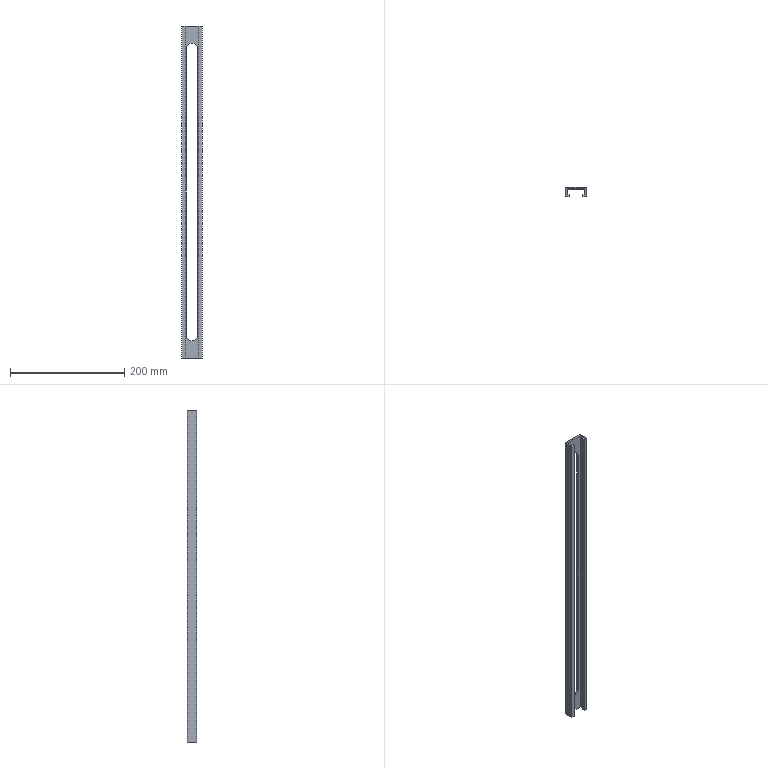Part | SolidWorks | features ICE 2, Extrusion 1 | 1 solid | 19 faces | box 36 x 16 x 580 mm | volume 87378 mm3 | plane 16 | cylinder 3 | commonest cylinder face diameters 20 x3
STEP:
#1=CARTESIAN_POINT('',(0.,13.,-260.));
#2=VERTEX_POINT('',#1);
#3=CARTESIAN_POINT('',(10.,13.,-250.));
#4=VERTEX_POINT('',#3);
#5=CARTESIAN_POINT('',(0.,13.,-250.));
#6=DIRECTION('',(0.,-1.,0.));
#7=DIRECTION('',(0.,0.,-1.));
#8=AXIS2_PLACEMENT_3D('',#5,#6,#7);
#9=CIRCLE('',#8,10.);
#10=EDGE_CURVE('',#2,#4,#9,.T.);
#11=ORIENTED_EDGE('',*,*,#10,.F.);
#12=CARTESIAN_POINT('',(0.,10.,-260.));
#13=VERTEX_POINT('',#12);
#14=CARTESIAN_POINT('',(0.,13.,-260.));
#15=DIRECTION('',(0.,-1.,0.));
#16=VECTOR('',#15,1000.);
#17=LINE('',#14,#16);
#18=EDGE_CURVE('',#2,#13,#17,.T.);
#19=ORIENTED_EDGE('',*,*,#18,.T.);
#20=CARTESIAN_POINT('',(10.,10.,-250.));
#21=VERTEX_POINT('',#20);
#22=CARTESIAN_POINT('',(0.,10.,-250.));
#23=DIRECTION('',(0.,-1.,0.));
#24=DIRECTION('',(0.,0.,-1.));
#25=AXIS2_PLACEMENT_3D('',#22,#23,#24);
#26=CIRCLE('',#25,10.);
#27=EDGE_CURVE('',#13,#21,#26,.T.);
#28=ORIENTED_EDGE('',*,*,#27,.T.);
#29=CARTESIAN_POINT('',(10.,13.,-250.));
#30=DIRECTION('',(0.,-1.,0.));
#31=VECTOR('',#30,1000.);
#32=LINE('',#29,#31);
#33=EDGE_CURVE('',#4,#21,#32,.T.);
#34=ORIENTED_EDGE('',*,*,#33,.F.);
#35=EDGE_LOOP('',(#11,#19,#28,#34));
#36=FACE_OUTER_BOUND('',#35,.T.);
#37=CARTESIAN_POINT('',(0.,13.,-250.));
#38=DIRECTION('',(0.,-1.,0.));
#39=DIRECTION('',(0.,0.,-1.));
#40=AXIS2_PLACEMENT_3D('',#37,#38,#39);
#41=CYLINDRICAL_SURFACE('',#40,10.);
#42=ADVANCED_FACE('',(#36),#41,.F.);
#43=CARTESIAN_POINT('',(12.,-3.,290.));
#44=VERTEX_POINT('',#43);
#45=CARTESIAN_POINT('',(18.,-3.,290.));
#46=VERTEX_POINT('',#45);
#47=CARTESIAN_POINT('',(-18.,-3.,290.));
#48=DIRECTION('',(1.,0.,0.));
#49=VECTOR('',#48,1000.);
#50=LINE('',#47,#49);
#51=EDGE_CURVE('',#44,#46,#50,.T.);
#52=ORIENTED_EDGE('',*,*,#51,.F.);
#53=CARTESIAN_POINT('',(12.,-3.,-290.));
#54=VERTEX_POINT('',#53);
#55=CARTESIAN_POINT('',(12.,-3.,290.));
#56=DIRECTION('',(0.,0.,-1.));
#57=VECTOR('',#56,1000.);
#58=LINE('',#55,#57);
#59=EDGE_CURVE('',#44,#54,#58,.T.);
#60=ORIENTED_EDGE('',*,*,#59,.T.);
#61=CARTESIAN_POINT('',(18.,-3.,-290.));
#62=VERTEX_POINT('',#61);
#63=CARTESIAN_POINT('',(18.,-3.,-290.));
#64=DIRECTION('',(-1.,0.,0.));
#65=VECTOR('',#64,1000.);
#66=LINE('',#63,#65);
#67=EDGE_CURVE('',#62,#54,#66,.T.);
#68=ORIENTED_EDGE('',*,*,#67,.F.);
#69=CARTESIAN_POINT('',(18.,-3.,290.));
#70=DIRECTION('',(0.,0.,-1.));
#71=VECTOR('',#70,1000.);
#72=LINE('',#69,#71);
#73=EDGE_CURVE('',#46,#62,#72,.T.);
#74=ORIENTED_EDGE('',*,*,#73,.F.);
#75=EDGE_LOOP('',(#52,#60,#68,#74));
#76=FACE_OUTER_BOUND('',#75,.T.);
#77=CARTESIAN_POINT('',(0.,-3.,0.));
#78=DIRECTION('',(0.,1.,0.));
#79=DIRECTION('',(0.,0.,1.));
#80=AXIS2_PLACEMENT_3D('',#77,#78,#79);
#81=PLANE('',#80);
#82=ADVANCED_FACE('',(#76),#81,.F.);
#83=CARTESIAN_POINT('',(-18.,13.,-290.));
#84=VERTEX_POINT('',#83);
#85=CARTESIAN_POINT('',(-18.,13.,290.));
#86=VERTEX_POINT('',#85);
#87=CARTESIAN_POINT('',(-18.,13.,-290.));
#88=DIRECTION('',(0.,0.,1.));
#89=VECTOR('',#88,1000.);
#90=LINE('',#87,#89);
#91=EDGE_CURVE('',#84,#86,#90,.T.);
#92=ORIENTED_EDGE('',*,*,#91,.F.);
#93=CARTESIAN_POINT('',(-18.,-3.,-290.));
#94=VERTEX_POINT('',#93);
#95=CARTESIAN_POINT('',(-18.,-3.,-290.));
#96=DIRECTION('',(0.,1.,0.));
#97=VECTOR('',#96,1000.);
#98=LINE('',#95,#97);
#99=EDGE_CURVE('',#94,#84,#98,.T.);
#100=ORIENTED_EDGE('',*,*,#99,.F.);
#101=CARTESIAN_POINT('',(-18.,-3.,290.));
#102=VERTEX_POINT('',#101);
#103=CARTESIAN_POINT('',(-18.,-3.,-290.));
#104=DIRECTION('',(0.,0.,1.));
#105=VECTOR('',#104,1000.);
#106=LINE('',#103,#105);
#107=EDGE_CURVE('',#94,#102,#106,.T.);
#108=ORIENTED_EDGE('',*,*,#107,.T.);
#109=CARTESIAN_POINT('',(-18.,-3.,290.));
#110=DIRECTION('',(0.,1.,0.));
#111=VECTOR('',#110,1000.);
#112=LINE('',#109,#111);
#113=EDGE_CURVE('',#102,#86,#112,.T.);
#114=ORIENTED_EDGE('',*,*,#113,.T.);
#115=EDGE_LOOP('',(#92,#100,#108,#114));
#116=FACE_OUTER_BOUND('',#115,.T.);
#117=CARTESIAN_POINT('',(-18.,-3.,-290.));
#118=DIRECTION('',(-1.,0.,0.));
#119=DIRECTION('',(0.,0.,1.));
#120=AXIS2_PLACEMENT_3D('',#117,#118,#119);
#121=PLANE('',#120);
#122=ADVANCED_FACE('',(#116),#121,.T.);
#123=CARTESIAN_POINT('',(12.,0.,-290.));
#124=VERTEX_POINT('',#123);
#125=CARTESIAN_POINT('',(12.,0.,-290.));
#126=DIRECTION('',(0.,-1.,0.));
#127=VECTOR('',#126,1000.);
#128=LINE('',#125,#127);
#129=EDGE_CURVE('',#124,#54,#128,.T.);
#130=ORIENTED_EDGE('',*,*,#129,.F.);
#131=CARTESIAN_POINT('',(15.,0.,-290.));
#132=VERTEX_POINT('',#131);
#133=CARTESIAN_POINT('',(15.,0.,-290.));
#134=DIRECTION('',(-1.,0.,0.));
#135=VECTOR('',#134,1000.);
#136=LINE('',#133,#135);
#137=EDGE_CURVE('',#132,#124,#136,.T.);
#138=ORIENTED_EDGE('',*,*,#137,.F.);
#139=CARTESIAN_POINT('',(15.,10.,-290.));
#140=VERTEX_POINT('',#139);
#141=CARTESIAN_POINT('',(15.,10.,-290.));
#142=DIRECTION('',(0.,-1.,0.));
#143=VECTOR('',#142,1000.);
#144=LINE('',#141,#143);
#145=EDGE_CURVE('',#140,#132,#144,.T.);
#146=ORIENTED_EDGE('',*,*,#145,.F.);
#147=CARTESIAN_POINT('',(-15.,10.,-290.));
#148=VERTEX_POINT('',#147);
#149=CARTESIAN_POINT('',(-15.,10.,-290.));
#150=DIRECTION('',(1.,0.,0.));
#151=VECTOR('',#150,1000.);
#152=LINE('',#149,#151);
#153=EDGE_CURVE('',#148,#140,#152,.T.);
#154=ORIENTED_EDGE('',*,*,#153,.F.);
#155=CARTESIAN_POINT('',(-15.,0.,-290.));
#156=VERTEX_POINT('',#155);
#157=CARTESIAN_POINT('',(-15.,0.,-290.));
#158=DIRECTION('',(0.,1.,0.));
#159=VECTOR('',#158,1000.);
#160=LINE('',#157,#159);
#161=EDGE_CURVE('',#156,#148,#160,.T.);
#162=ORIENTED_EDGE('',*,*,#161,.F.);
#163=CARTESIAN_POINT('',(-12.,0.,-290.));
#164=VERTEX_POINT('',#163);
#165=CARTESIAN_POINT('',(-12.,0.,-290.));
#166=DIRECTION('',(-1.,0.,0.));
#167=VECTOR('',#166,1000.);
#168=LINE('',#165,#167);
#169=EDGE_CURVE('',#164,#156,#168,.T.);
#170=ORIENTED_EDGE('',*,*,#169,.F.);
#171=CARTESIAN_POINT('',(-12.,-3.,-290.));
#172=VERTEX_POINT('',#171);
#173=CARTESIAN_POINT('',(-12.,-3.,-290.));
#174=DIRECTION('',(0.,1.,0.));
#175=VECTOR('',#174,1000.);
#176=LINE('',#173,#175);
#177=EDGE_CURVE('',#172,#164,#176,.T.);
#178=ORIENTED_EDGE('',*,*,#177,.F.);
#179=CARTESIAN_POINT('',(18.,-3.,-290.));
#180=DIRECTION('',(-1.,0.,0.));
#181=VECTOR('',#180,1000.);
#182=LINE('',#179,#181);
#183=EDGE_CURVE('',#172,#94,#182,.T.);
#184=ORIENTED_EDGE('',*,*,#183,.T.);
#185=ORIENTED_EDGE('',*,*,#99,.T.);
#186=CARTESIAN_POINT('',(18.,13.,-290.));
#187=VERTEX_POINT('',#186);
#188=CARTESIAN_POINT('',(18.,13.,-290.));
#189=DIRECTION('',(-1.,0.,0.));
#190=VECTOR('',#189,1000.);
#191=LINE('',#188,#190);
#192=EDGE_CURVE('',#187,#84,#191,.T.);
#193=ORIENTED_EDGE('',*,*,#192,.F.);
#194=CARTESIAN_POINT('',(18.,-3.,-290.));
#195=DIRECTION('',(0.,1.,0.));
#196=VECTOR('',#195,1000.);
#197=LINE('',#194,#196);
#198=EDGE_CURVE('',#62,#187,#197,.T.);
#199=ORIENTED_EDGE('',*,*,#198,.F.);
#200=ORIENTED_EDGE('',*,*,#67,.T.);
#201=EDGE_LOOP('',(#130,#138,#146,#154,#162,#170,#178,#184,#185,#193,#199,#200));
#202=FACE_OUTER_BOUND('',#201,.T.);
#203=CARTESIAN_POINT('',(18.,-3.,-290.));
#204=DIRECTION('',(0.,0.,-1.));
#205=DIRECTION('',(-1.,0.,0.));
#206=AXIS2_PLACEMENT_3D('',#203,#204,#205);
#207=PLANE('',#206);
#208=ADVANCED_FACE('',(#202),#207,.T.);
#209=CARTESIAN_POINT('',(18.,13.,290.));
#210=VERTEX_POINT('',#209);
#211=CARTESIAN_POINT('',(18.,13.,290.));
#212=DIRECTION('',(0.,0.,-1.));
#213=VECTOR('',#212,1000.);
#214=LINE('',#211,#213);
#215=EDGE_CURVE('',#210,#187,#214,.T.);
#216=ORIENTED_EDGE('',*,*,#215,.F.);
#217=CARTESIAN_POINT('',(18.,-3.,290.));
#218=DIRECTION('',(0.,1.,0.));
#219=VECTOR('',#218,1000.);
#220=LINE('',#217,#219);
#221=EDGE_CURVE('',#46,#210,#220,.T.);
#222=ORIENTED_EDGE('',*,*,#221,.F.);
#223=ORIENTED_EDGE('',*,*,#73,.T.);
#224=ORIENTED_EDGE('',*,*,#198,.T.);
#225=EDGE_LOOP('',(#216,#222,#223,#224));
#226=FACE_OUTER_BOUND('',#225,.T.);
#227=CARTESIAN_POINT('',(18.,-3.,290.));
#228=DIRECTION('',(1.,0.,0.));
#229=DIRECTION('',(0.,0.,-1.));
#230=AXIS2_PLACEMENT_3D('',#227,#228,#229);
#231=PLANE('',#230);
#232=ADVANCED_FACE('',(#226),#231,.T.);
#233=CARTESIAN_POINT('',(12.,0.,290.));
#234=VERTEX_POINT('',#233);
#235=CARTESIAN_POINT('',(12.,0.,290.));
#236=DIRECTION('',(0.,-1.,0.));
#237=VECTOR('',#236,1000.);
#238=LINE('',#235,#237);
#239=EDGE_CURVE('',#234,#44,#238,.T.);
#240=ORIENTED_EDGE('',*,*,#239,.T.);
#241=ORIENTED_EDGE('',*,*,#51,.T.);
#242=ORIENTED_EDGE('',*,*,#221,.T.);
#243=CARTESIAN_POINT('',(-18.,13.,290.));
#244=DIRECTION('',(1.,0.,0.));
#245=VECTOR('',#244,1000.);
#246=LINE('',#243,#245);
#247=EDGE_CURVE('',#86,#210,#246,.T.);
#248=ORIENTED_EDGE('',*,*,#247,.F.);
#249=ORIENTED_EDGE('',*,*,#113,.F.);
#250=CARTESIAN_POINT('',(-12.,-3.,290.));
#251=VERTEX_POINT('',#250);
#252=CARTESIAN_POINT('',(-18.,-3.,290.));
#253=DIRECTION('',(1.,0.,0.));
#254=VECTOR('',#253,1000.);
#255=LINE('',#252,#254);
#256=EDGE_CURVE('',#102,#251,#255,.T.);
#257=ORIENTED_EDGE('',*,*,#256,.T.);
#258=CARTESIAN_POINT('',(-12.,0.,290.));
#259=VERTEX_POINT('',#258);
#260=CARTESIAN_POINT('',(-12.,-3.,290.));
#261=DIRECTION('',(0.,1.,0.));
#262=VECTOR('',#261,1000.);
#263=LINE('',#260,#262);
#264=EDGE_CURVE('',#251,#259,#263,.T.);
#265=ORIENTED_EDGE('',*,*,#264,.T.);
#266=CARTESIAN_POINT('',(-15.,0.,290.));
#267=VERTEX_POINT('',#266);
#268=CARTESIAN_POINT('',(-12.,0.,290.));
#269=DIRECTION('',(-1.,0.,0.));
#270=VECTOR('',#269,1000.);
#271=LINE('',#268,#270);
#272=EDGE_CURVE('',#259,#267,#271,.T.);
#273=ORIENTED_EDGE('',*,*,#272,.T.);
#274=CARTESIAN_POINT('',(-15.,10.,290.));
#275=VERTEX_POINT('',#274);
#276=CARTESIAN_POINT('',(-15.,0.,290.));
#277=DIRECTION('',(0.,1.,0.));
#278=VECTOR('',#277,1000.);
#279=LINE('',#276,#278);
#280=EDGE_CURVE('',#267,#275,#279,.T.);
#281=ORIENTED_EDGE('',*,*,#280,.T.);
#282=CARTESIAN_POINT('',(15.,10.,290.));
#283=VERTEX_POINT('',#282);
#284=CARTESIAN_POINT('',(-15.,10.,290.));
#285=DIRECTION('',(1.,0.,0.));
#286=VECTOR('',#285,1000.);
#287=LINE('',#284,#286);
#288=EDGE_CURVE('',#275,#283,#287,.T.);
#289=ORIENTED_EDGE('',*,*,#288,.T.);
#290=CARTESIAN_POINT('',(15.,0.,290.));
#291=VERTEX_POINT('',#290);
#292=CARTESIAN_POINT('',(15.,10.,290.));
#293=DIRECTION('',(0.,-1.,0.));
#294=VECTOR('',#293,1000.);
#295=LINE('',#292,#294);
#296=EDGE_CURVE('',#283,#291,#295,.T.);
#297=ORIENTED_EDGE('',*,*,#296,.T.);
#298=CARTESIAN_POINT('',(15.,0.,290.));
#299=DIRECTION('',(-1.,0.,0.));
#300=VECTOR('',#299,1000.);
#301=LINE('',#298,#300);
#302=EDGE_CURVE('',#291,#234,#301,.T.);
#303=ORIENTED_EDGE('',*,*,#302,.T.);
#304=EDGE_LOOP('',(#240,#241,#242,#248,#249,#257,#265,#273,#281,#289,#297,#303));
#305=FACE_OUTER_BOUND('',#304,.T.);
#306=CARTESIAN_POINT('',(-18.,-3.,290.));
#307=DIRECTION('',(0.,0.,1.));
#308=DIRECTION('',(1.,0.,0.));
#309=AXIS2_PLACEMENT_3D('',#306,#307,#308);
#310=PLANE('',#309);
#311=ADVANCED_FACE('',(#305),#310,.T.);
#312=ORIENTED_EDGE('',*,*,#183,.F.);
#313=CARTESIAN_POINT('',(-12.,-3.,290.));
#314=DIRECTION('',(0.,0.,-1.));
#315=VECTOR('',#314,1000.);
#316=LINE('',#313,#315);
#317=EDGE_CURVE('',#251,#172,#316,.T.);
#318=ORIENTED_EDGE('',*,*,#317,.F.);
#319=ORIENTED_EDGE('',*,*,#256,.F.);
#320=ORIENTED_EDGE('',*,*,#107,.F.);
#321=EDGE_LOOP('',(#312,#318,#319,#320));
#322=FACE_OUTER_BOUND('',#321,.T.);
#323=CARTESIAN_POINT('',(0.,-3.,0.));
#324=DIRECTION('',(0.,1.,0.));
#325=DIRECTION('',(0.,0.,1.));
#326=AXIS2_PLACEMENT_3D('',#323,#324,#325);
#327=PLANE('',#326);
#328=ADVANCED_FACE('',(#322),#327,.F.);
#329=CARTESIAN_POINT('',(-10.,13.,-250.));
#330=VERTEX_POINT('',#329);
#331=CARTESIAN_POINT('',(0.,13.,-250.));
#332=DIRECTION('',(0.,-1.,0.));
#333=DIRECTION('',(0.,0.,-1.));
#334=AXIS2_PLACEMENT_3D('',#331,#332,#333);
#335=CIRCLE('',#334,10.);
#336=EDGE_CURVE('',#330,#2,#335,.T.);
#337=ORIENTED_EDGE('',*,*,#336,.T.);
#338=ORIENTED_EDGE('',*,*,#10,.T.);
#339=CARTESIAN_POINT('',(10.,13.,250.));
#340=VERTEX_POINT('',#339);
#341=CARTESIAN_POINT('',(10.,13.,-250.));
#342=DIRECTION('',(0.,0.,1.));
#343=VECTOR('',#342,1000.);
#344=LINE('',#341,#343);
#345=EDGE_CURVE('',#4,#340,#344,.T.);
#346=ORIENTED_EDGE('',*,*,#345,.T.);
#347=CARTESIAN_POINT('',(-10.,13.,250.));
#348=VERTEX_POINT('',#347);
#349=CARTESIAN_POINT('',(0.,13.,250.));
#350=DIRECTION('',(0.,-1.,0.));
#351=DIRECTION('',(0.,0.,-1.));
#352=AXIS2_PLACEMENT_3D('',#349,#350,#351);
#353=CIRCLE('',#352,10.);
#354=EDGE_CURVE('',#340,#348,#353,.T.);
#355=ORIENTED_EDGE('',*,*,#354,.T.);
#356=CARTESIAN_POINT('',(-10.,13.,250.));
#357=DIRECTION('',(0.,0.,-1.));
#358=VECTOR('',#357,1000.);
#359=LINE('',#356,#358);
#360=EDGE_CURVE('',#348,#330,#359,.T.);
#361=ORIENTED_EDGE('',*,*,#360,.T.);
#362=EDGE_LOOP('',(#337,#338,#346,#355,#361));
#363=FACE_BOUND('',#362,.T.);
#364=ORIENTED_EDGE('',*,*,#91,.T.);
#365=ORIENTED_EDGE('',*,*,#247,.T.);
#366=ORIENTED_EDGE('',*,*,#215,.T.);
#367=ORIENTED_EDGE('',*,*,#192,.T.);
#368=EDGE_LOOP('',(#364,#365,#366,#367));
#369=FACE_OUTER_BOUND('',#368,.T.);
#370=CARTESIAN_POINT('',(0.,13.,0.));
#371=DIRECTION('',(0.,1.,0.));
#372=DIRECTION('',(0.,0.,1.));
#373=AXIS2_PLACEMENT_3D('',#370,#371,#372);
#374=PLANE('',#373);
#375=ADVANCED_FACE('',(#363,#369),#374,.T.);
#376=ORIENTED_EDGE('',*,*,#129,.T.);
#377=ORIENTED_EDGE('',*,*,#59,.F.);
#378=ORIENTED_EDGE('',*,*,#239,.F.);
#379=CARTESIAN_POINT('',(12.,0.,290.));
#380=DIRECTION('',(0.,0.,-1.));
#381=VECTOR('',#380,1000.);
#382=LINE('',#379,#381);
#383=EDGE_CURVE('',#234,#124,#382,.T.);
#384=ORIENTED_EDGE('',*,*,#383,.T.);
#385=EDGE_LOOP('',(#376,#377,#378,#384));
#386=FACE_OUTER_BOUND('',#385,.T.);
#387=CARTESIAN_POINT('',(12.,0.,290.));
#388=DIRECTION('',(1.,0.,0.));
#389=DIRECTION('',(0.,0.,-1.));
#390=AXIS2_PLACEMENT_3D('',#387,#388,#389);
#391=PLANE('',#390);
#392=ADVANCED_FACE('',(#386),#391,.F.);
#393=ORIENTED_EDGE('',*,*,#137,.T.);
#394=ORIENTED_EDGE('',*,*,#383,.F.);
#395=ORIENTED_EDGE('',*,*,#302,.F.);
#396=CARTESIAN_POINT('',(15.,0.,290.));
#397=DIRECTION('',(0.,0.,-1.));
#398=VECTOR('',#397,1000.);
#399=LINE('',#396,#398);
#400=EDGE_CURVE('',#291,#132,#399,.T.);
#401=ORIENTED_EDGE('',*,*,#400,.T.);
#402=EDGE_LOOP('',(#393,#394,#395,#401));
#403=FACE_OUTER_BOUND('',#402,.T.);
#404=CARTESIAN_POINT('',(15.,0.,290.));
#405=DIRECTION('',(0.,-1.,0.));
#406=DIRECTION('',(0.,0.,-1.));
#407=AXIS2_PLACEMENT_3D('',#404,#405,#406);
#408=PLANE('',#407);
#409=ADVANCED_FACE('',(#403),#408,.F.);
#410=ORIENTED_EDGE('',*,*,#145,.T.);
#411=ORIENTED_EDGE('',*,*,#400,.F.);
#412=ORIENTED_EDGE('',*,*,#296,.F.);
#413=CARTESIAN_POINT('',(15.,10.,290.));
#414=DIRECTION('',(0.,0.,-1.));
#415=VECTOR('',#414,1000.);
#416=LINE('',#413,#415);
#417=EDGE_CURVE('',#283,#140,#416,.T.);
#418=ORIENTED_EDGE('',*,*,#417,.T.);
#419=EDGE_LOOP('',(#410,#411,#412,#418));
#420=FACE_OUTER_BOUND('',#419,.T.);
#421=CARTESIAN_POINT('',(15.,10.,290.));
#422=DIRECTION('',(1.,0.,0.));
#423=DIRECTION('',(0.,0.,-1.));
#424=AXIS2_PLACEMENT_3D('',#421,#422,#423);
#425=PLANE('',#424);
#426=ADVANCED_FACE('',(#420),#425,.F.);
#427=CARTESIAN_POINT('',(10.,10.,250.));
#428=VERTEX_POINT('',#427);
#429=CARTESIAN_POINT('',(10.,10.,-250.));
#430=DIRECTION('',(0.,0.,1.));
#431=VECTOR('',#430,1000.);
#432=LINE('',#429,#431);
#433=EDGE_CURVE('',#21,#428,#432,.T.);
#434=ORIENTED_EDGE('',*,*,#433,.F.);
#435=ORIENTED_EDGE('',*,*,#27,.F.);
#436=CARTESIAN_POINT('',(-10.,10.,-250.));
#437=VERTEX_POINT('',#436);
#438=CARTESIAN_POINT('',(0.,10.,-250.));
#439=DIRECTION('',(0.,-1.,0.));
#440=DIRECTION('',(0.,0.,-1.));
#441=AXIS2_PLACEMENT_3D('',#438,#439,#440);
#442=CIRCLE('',#441,10.);
#443=EDGE_CURVE('',#437,#13,#442,.T.);
#444=ORIENTED_EDGE('',*,*,#443,.F.);
#445=CARTESIAN_POINT('',(-10.,10.,250.));
#446=VERTEX_POINT('',#445);
#447=CARTESIAN_POINT('',(-10.,10.,250.));
#448=DIRECTION('',(0.,0.,-1.));
#449=VECTOR('',#448,1000.);
#450=LINE('',#447,#449);
#451=EDGE_CURVE('',#446,#437,#450,.T.);
#452=ORIENTED_EDGE('',*,*,#451,.F.);
#453=CARTESIAN_POINT('',(0.,10.,250.));
#454=DIRECTION('',(0.,-1.,0.));
#455=DIRECTION('',(0.,0.,-1.));
#456=AXIS2_PLACEMENT_3D('',#453,#454,#455);
#457=CIRCLE('',#456,10.);
#458=EDGE_CURVE('',#428,#446,#457,.T.);
#459=ORIENTED_EDGE('',*,*,#458,.F.);
#460=EDGE_LOOP('',(#434,#435,#444,#452,#459));
#461=FACE_BOUND('',#460,.T.);
#462=ORIENTED_EDGE('',*,*,#153,.T.);
#463=ORIENTED_EDGE('',*,*,#417,.F.);
#464=ORIENTED_EDGE('',*,*,#288,.F.);
#465=CARTESIAN_POINT('',(-15.,10.,290.));
#466=DIRECTION('',(0.,0.,-1.));
#467=VECTOR('',#466,1000.);
#468=LINE('',#465,#467);
#469=EDGE_CURVE('',#275,#148,#468,.T.);
#470=ORIENTED_EDGE('',*,*,#469,.T.);
#471=EDGE_LOOP('',(#462,#463,#464,#470));
#472=FACE_OUTER_BOUND('',#471,.T.);
#473=CARTESIAN_POINT('',(-15.,10.,290.));
#474=DIRECTION('',(0.,1.,0.));
#475=DIRECTION('',(0.,0.,1.));
#476=AXIS2_PLACEMENT_3D('',#473,#474,#475);
#477=PLANE('',#476);
#478=ADVANCED_FACE('',(#461,#472),#477,.F.);
#479=ORIENTED_EDGE('',*,*,#161,.T.);
#480=ORIENTED_EDGE('',*,*,#469,.F.);
#481=ORIENTED_EDGE('',*,*,#280,.F.);
#482=CARTESIAN_POINT('',(-15.,0.,290.));
#483=DIRECTION('',(0.,0.,-1.));
#484=VECTOR('',#483,1000.);
#485=LINE('',#482,#484);
#486=EDGE_CURVE('',#267,#156,#485,.T.);
#487=ORIENTED_EDGE('',*,*,#486,.T.);
#488=EDGE_LOOP('',(#479,#480,#481,#487));
#489=FACE_OUTER_BOUND('',#488,.T.);
#490=CARTESIAN_POINT('',(-15.,0.,290.));
#491=DIRECTION('',(-1.,0.,0.));
#492=DIRECTION('',(0.,0.,1.));
#493=AXIS2_PLACEMENT_3D('',#490,#491,#492);
#494=PLANE('',#493);
#495=ADVANCED_FACE('',(#489),#494,.F.);
#496=ORIENTED_EDGE('',*,*,#169,.T.);
#497=ORIENTED_EDGE('',*,*,#486,.F.);
#498=ORIENTED_EDGE('',*,*,#272,.F.);
#499=CARTESIAN_POINT('',(-12.,0.,290.));
#500=DIRECTION('',(0.,0.,-1.));
#501=VECTOR('',#500,1000.);
#502=LINE('',#499,#501);
#503=EDGE_CURVE('',#259,#164,#502,.T.);
#504=ORIENTED_EDGE('',*,*,#503,.T.);
#505=EDGE_LOOP('',(#496,#497,#498,#504));
#506=FACE_OUTER_BOUND('',#505,.T.);
#507=CARTESIAN_POINT('',(-12.,0.,290.));
#508=DIRECTION('',(0.,-1.,0.));
#509=DIRECTION('',(0.,0.,-1.));
#510=AXIS2_PLACEMENT_3D('',#507,#508,#509);
#511=PLANE('',#510);
#512=ADVANCED_FACE('',(#506),#511,.F.);
#513=ORIENTED_EDGE('',*,*,#177,.T.);
#514=ORIENTED_EDGE('',*,*,#503,.F.);
#515=ORIENTED_EDGE('',*,*,#264,.F.);
#516=ORIENTED_EDGE('',*,*,#317,.T.);
#517=EDGE_LOOP('',(#513,#514,#515,#516));
#518=FACE_OUTER_BOUND('',#517,.T.);
#519=CARTESIAN_POINT('',(-12.,-3.,290.));
#520=DIRECTION('',(-1.,0.,0.));
#521=DIRECTION('',(0.,0.,1.));
#522=AXIS2_PLACEMENT_3D('',#519,#520,#521);
#523=PLANE('',#522);
#524=ADVANCED_FACE('',(#518),#523,.F.);
#525=ORIENTED_EDGE('',*,*,#18,.F.);
#526=ORIENTED_EDGE('',*,*,#336,.F.);
#527=CARTESIAN_POINT('',(-10.,13.,-250.));
#528=DIRECTION('',(0.,-1.,0.));
#529=VECTOR('',#528,1000.);
#530=LINE('',#527,#529);
#531=EDGE_CURVE('',#330,#437,#530,.T.);
#532=ORIENTED_EDGE('',*,*,#531,.T.);
#533=ORIENTED_EDGE('',*,*,#443,.T.);
#534=EDGE_LOOP('',(#525,#526,#532,#533));
#535=FACE_OUTER_BOUND('',#534,.T.);
#536=CARTESIAN_POINT('',(0.,13.,-250.));
#537=DIRECTION('',(0.,-1.,0.));
#538=DIRECTION('',(0.,0.,-1.));
#539=AXIS2_PLACEMENT_3D('',#536,#537,#538);
#540=CYLINDRICAL_SURFACE('',#539,10.);
#541=ADVANCED_FACE('',(#535),#540,.F.);
#542=ORIENTED_EDGE('',*,*,#451,.T.);
#543=ORIENTED_EDGE('',*,*,#531,.F.);
#544=ORIENTED_EDGE('',*,*,#360,.F.);
#545=CARTESIAN_POINT('',(-10.,13.,250.));
#546=DIRECTION('',(0.,-1.,0.));
#547=VECTOR('',#546,1000.);
#548=LINE('',#545,#547);
#549=EDGE_CURVE('',#348,#446,#548,.T.);
#550=ORIENTED_EDGE('',*,*,#549,.T.);
#551=EDGE_LOOP('',(#542,#543,#544,#550));
#552=FACE_OUTER_BOUND('',#551,.T.);
#553=CARTESIAN_POINT('',(-10.,13.,250.));
#554=DIRECTION('',(-1.,0.,0.));
#555=DIRECTION('',(0.,0.,1.));
#556=AXIS2_PLACEMENT_3D('',#553,#554,#555);
#557=PLANE('',#556);
#558=ADVANCED_FACE('',(#552),#557,.F.);
#559=ORIENTED_EDGE('',*,*,#458,.T.);
#560=ORIENTED_EDGE('',*,*,#549,.F.);
#561=ORIENTED_EDGE('',*,*,#354,.F.);
#562=CARTESIAN_POINT('',(10.,13.,250.));
#563=DIRECTION('',(0.,-1.,0.));
#564=VECTOR('',#563,1000.);
#565=LINE('',#562,#564);
#566=EDGE_CURVE('',#340,#428,#565,.T.);
#567=ORIENTED_EDGE('',*,*,#566,.T.);
#568=EDGE_LOOP('',(#559,#560,#561,#567));
#569=FACE_OUTER_BOUND('',#568,.T.);
#570=CARTESIAN_POINT('',(0.,13.,250.));
#571=DIRECTION('',(0.,-1.,0.));
#572=DIRECTION('',(0.,0.,-1.));
#573=AXIS2_PLACEMENT_3D('',#570,#571,#572);
#574=CYLINDRICAL_SURFACE('',#573,10.);
#575=ADVANCED_FACE('',(#569),#574,.F.);
#576=ORIENTED_EDGE('',*,*,#433,.T.);
#577=ORIENTED_EDGE('',*,*,#566,.F.);
#578=ORIENTED_EDGE('',*,*,#345,.F.);
#579=ORIENTED_EDGE('',*,*,#33,.T.);
#580=EDGE_LOOP('',(#576,#577,#578,#579));
#581=FACE_OUTER_BOUND('',#580,.T.);
#582=CARTESIAN_POINT('',(10.,13.,-250.));
#583=DIRECTION('',(1.,0.,0.));
#584=DIRECTION('',(0.,0.,-1.));
#585=AXIS2_PLACEMENT_3D('',#582,#583,#584);
#586=PLANE('',#585);
#587=ADVANCED_FACE('',(#581),#586,.F.);
#588=CLOSED_SHELL('',(#42,#82,#122,#208,#232,#311,#328,#375,#392,#409,#426,#478,#495,#512,#524,#541,#558,#575,#587));
#589=MANIFOLD_SOLID_BREP('',#588);
#590=CARTESIAN_POINT('',(0.,0.,0.));
#591=DIRECTION('',(0.,0.,1.));
#592=DIRECTION('',(1.,0.,0.));
#593=AXIS2_PLACEMENT_3D('',#590,#591,#592);
#594=(LENGTH_UNIT()NAMED_UNIT(*)SI_UNIT(.MILLI.,.METRE.));
#595=UNCERTAINTY_MEASURE_WITH_UNIT(LENGTH_MEASURE(0.00001),#594,'','');
#596=(NAMED_UNIT(*)PLANE_ANGLE_UNIT()SI_UNIT($,.RADIAN.));
#597=(NAMED_UNIT(*)SI_UNIT($,.STERADIAN.)SOLID_ANGLE_UNIT());
#598=(GEOMETRIC_REPRESENTATION_CONTEXT(3)GLOBAL_UNCERTAINTY_ASSIGNED_CONTEXT((#595))GLOBAL_UNIT_ASSIGNED_CONTEXT((#594,#596,#597))REPRESENTATION_CONTEXT('',''));
#599=ADVANCED_BREP_SHAPE_REPRESENTATION('',(#589,#593),#598);